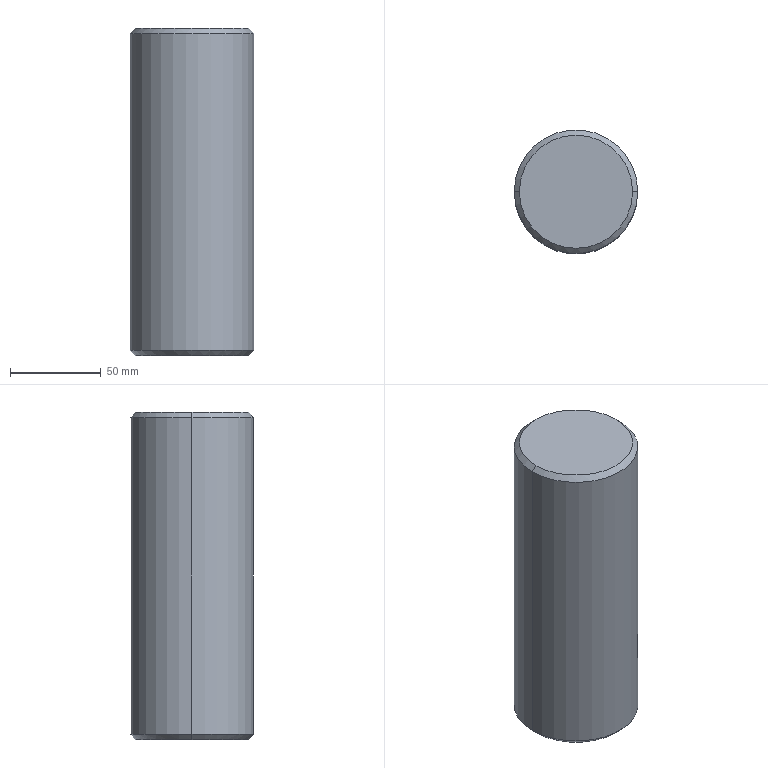Part | SolidWorks | features BaseBody 1 | 1 solid | 12 faces | box 68 x 68 x 180 mm | volume 648919 mm3 | cone 6 | cylinder 4 | plane 2 | commonest cylinder face diameters 10.5 x2 68 x2
STEP:
#1=CARTESIAN_POINT('',(214.75,-51.999,-390.5));
#2=VERTEX_POINT('',#1);
#3=CARTESIAN_POINT('',(225.25,-51.999,-390.5));
#4=VERTEX_POINT('',#3);
#5=CARTESIAN_POINT('',(220.,-51.999,-390.5));
#6=DIRECTION('',(0.,0.,1.));
#7=DIRECTION('',(1.,0.,0.));
#8=AXIS2_PLACEMENT_3D('',#5,#6,#7);
#9=CIRCLE('',#8,5.25);
#10=EDGE_CURVE('',#2,#4,#9,.T.);
#11=ORIENTED_EDGE('',*,*,#10,.F.);
#12=CARTESIAN_POINT('',(214.75,-51.999,-355.5));
#13=VERTEX_POINT('',#12);
#14=CARTESIAN_POINT('',(214.75,-51.999,-390.5));
#15=DIRECTION('',(0.,0.,1.));
#16=VECTOR('',#15,1000.);
#17=LINE('',#14,#16);
#18=EDGE_CURVE('',#2,#13,#17,.T.);
#19=ORIENTED_EDGE('',*,*,#18,.T.);
#20=CARTESIAN_POINT('',(225.25,-51.999,-355.5));
#21=VERTEX_POINT('',#20);
#22=CARTESIAN_POINT('',(220.,-51.999,-355.5));
#23=DIRECTION('',(0.,0.,1.));
#24=DIRECTION('',(1.,0.,0.));
#25=AXIS2_PLACEMENT_3D('',#22,#23,#24);
#26=CIRCLE('',#25,5.25);
#27=EDGE_CURVE('',#13,#21,#26,.T.);
#28=ORIENTED_EDGE('',*,*,#27,.T.);
#29=CARTESIAN_POINT('',(225.25,-51.999,-390.5));
#30=DIRECTION('',(0.,0.,1.));
#31=VECTOR('',#30,1000.);
#32=LINE('',#29,#31);
#33=EDGE_CURVE('',#4,#21,#32,.T.);
#34=ORIENTED_EDGE('',*,*,#33,.F.);
#35=EDGE_LOOP('',(#11,#19,#28,#34));
#36=FACE_OUTER_BOUND('',#35,.T.);
#37=CARTESIAN_POINT('',(220.,-51.999,-390.5));
#38=DIRECTION('',(0.,0.,1.));
#39=DIRECTION('',(1.,0.,0.));
#40=AXIS2_PLACEMENT_3D('',#37,#38,#39);
#41=CYLINDRICAL_SURFACE('',#40,5.25);
#42=ADVANCED_FACE('',(#36),#41,.F.);
#43=CARTESIAN_POINT('',(220.,-51.999,-352.345));
#44=VERTEX_POINT('',#43);
#45=CARTESIAN_POINT('',(214.75,-51.999,-355.5));
#46=DIRECTION('',(-0.8572,0.,-0.515));
#47=VECTOR('',#46,1000.);
#48=LINE('',#45,#47);
#49=EDGE_CURVE('',#44,#13,#48,.T.);
#50=ORIENTED_EDGE('',*,*,#49,.F.);
#51=CARTESIAN_POINT('',(225.25,-51.999,-355.5));
#52=DIRECTION('',(0.8572,0.,-0.515));
#53=VECTOR('',#52,1000.);
#54=LINE('',#51,#53);
#55=EDGE_CURVE('',#44,#21,#54,.T.);
#56=ORIENTED_EDGE('',*,*,#55,.T.);
#57=ORIENTED_EDGE('',*,*,#27,.F.);
#58=EDGE_LOOP('',(#50,#56,#57));
#59=FACE_OUTER_BOUND('',#58,.T.);
#60=CARTESIAN_POINT('',(220.,-51.999,-355.5));
#61=DIRECTION('',(0.,0.,-1.));
#62=DIRECTION('',(-1.,0.,0.));
#63=AXIS2_PLACEMENT_3D('',#60,#61,#62);
#64=CONICAL_SURFACE('',#63,5.25,1.03);
#65=ADVANCED_FACE('',(#59),#64,.F.);
#66=CARTESIAN_POINT('',(251.172,-51.999,-210.5));
#67=VERTEX_POINT('',#66);
#68=CARTESIAN_POINT('',(188.828,-51.999,-210.5));
#69=VERTEX_POINT('',#68);
#70=CARTESIAN_POINT('',(220.,-51.999,-210.5));
#71=DIRECTION('',(0.,0.,1.));
#72=DIRECTION('',(1.,0.,0.));
#73=AXIS2_PLACEMENT_3D('',#70,#71,#72);
#74=CIRCLE('',#73,31.172);
#75=EDGE_CURVE('',#67,#69,#74,.T.);
#76=ORIENTED_EDGE('',*,*,#75,.F.);
#77=CARTESIAN_POINT('',(254.,-51.999,-213.328));
#78=VERTEX_POINT('',#77);
#79=CARTESIAN_POINT('',(252.586,-51.999,-211.914));
#80=DIRECTION('',(0.7071,0.,-0.7071));
#81=VECTOR('',#80,1000.);
#82=LINE('',#79,#81);
#83=EDGE_CURVE('',#67,#78,#82,.T.);
#84=ORIENTED_EDGE('',*,*,#83,.T.);
#85=CARTESIAN_POINT('',(186.,-51.999,-213.328));
#86=VERTEX_POINT('',#85);
#87=CARTESIAN_POINT('',(220.,-51.999,-213.328));
#88=DIRECTION('',(0.,0.,-1.));
#89=DIRECTION('',(-1.,0.,0.));
#90=AXIS2_PLACEMENT_3D('',#87,#88,#89);
#91=CIRCLE('',#90,34.);
#92=EDGE_CURVE('',#86,#78,#91,.T.);
#93=ORIENTED_EDGE('',*,*,#92,.F.);
#94=CARTESIAN_POINT('',(187.414,-51.999,-211.914));
#95=DIRECTION('',(-0.7071,0.,-0.7071));
#96=VECTOR('',#95,1000.);
#97=LINE('',#94,#96);
#98=EDGE_CURVE('',#69,#86,#97,.T.);
#99=ORIENTED_EDGE('',*,*,#98,.F.);
#100=EDGE_LOOP('',(#76,#84,#93,#99));
#101=FACE_OUTER_BOUND('',#100,.T.);
#102=CARTESIAN_POINT('',(220.,-51.999,-211.914));
#103=DIRECTION('',(0.,0.,-1.));
#104=DIRECTION('',(-1.,0.,0.));
#105=AXIS2_PLACEMENT_3D('',#102,#103,#104);
#106=CONICAL_SURFACE('',#105,32.586,0.7854);
#107=ADVANCED_FACE('',(#101),#106,.T.);
#108=CARTESIAN_POINT('',(188.828,-51.999,-390.5));
#109=VERTEX_POINT('',#108);
#110=CARTESIAN_POINT('',(251.172,-51.999,-390.5));
#111=VERTEX_POINT('',#110);
#112=CARTESIAN_POINT('',(220.,-51.999,-390.5));
#113=DIRECTION('',(0.,0.,-1.));
#114=DIRECTION('',(1.,0.,0.));
#115=AXIS2_PLACEMENT_3D('',#112,#113,#114);
#116=CIRCLE('',#115,31.172);
#117=EDGE_CURVE('',#109,#111,#116,.T.);
#118=ORIENTED_EDGE('',*,*,#117,.F.);
#119=CARTESIAN_POINT('',(186.,-51.999,-387.672));
#120=VERTEX_POINT('',#119);
#121=CARTESIAN_POINT('',(185.414,-51.999,-387.086));
#122=DIRECTION('',(-0.7071,0.,0.7071));
#123=VECTOR('',#122,1000.);
#124=LINE('',#121,#123);
#125=EDGE_CURVE('',#109,#120,#124,.T.);
#126=ORIENTED_EDGE('',*,*,#125,.T.);
#127=CARTESIAN_POINT('',(254.,-51.999,-387.672));
#128=VERTEX_POINT('',#127);
#129=CARTESIAN_POINT('',(220.,-51.999,-387.672));
#130=DIRECTION('',(0.,0.,1.));
#131=DIRECTION('',(1.,0.,0.));
#132=AXIS2_PLACEMENT_3D('',#129,#130,#131);
#133=CIRCLE('',#132,34.);
#134=EDGE_CURVE('',#128,#120,#133,.T.);
#135=ORIENTED_EDGE('',*,*,#134,.F.);
#136=CARTESIAN_POINT('',(254.586,-51.999,-387.086));
#137=DIRECTION('',(0.7071,0.,0.7071));
#138=VECTOR('',#137,1000.);
#139=LINE('',#136,#138);
#140=EDGE_CURVE('',#111,#128,#139,.T.);
#141=ORIENTED_EDGE('',*,*,#140,.F.);
#142=EDGE_LOOP('',(#118,#126,#135,#141));
#143=FACE_OUTER_BOUND('',#142,.T.);
#144=CARTESIAN_POINT('',(220.,-51.999,-387.086));
#145=DIRECTION('',(0.,0.,1.));
#146=DIRECTION('',(1.,0.,0.));
#147=AXIS2_PLACEMENT_3D('',#144,#145,#146);
#148=CONICAL_SURFACE('',#147,34.586,0.7854);
#149=ADVANCED_FACE('',(#143),#148,.T.);
#150=ORIENTED_EDGE('',*,*,#92,.T.);
#151=CARTESIAN_POINT('',(254.,-51.999,-210.5));
#152=DIRECTION('',(0.,0.,-1.));
#153=VECTOR('',#152,1000.);
#154=LINE('',#151,#153);
#155=EDGE_CURVE('',#78,#128,#154,.T.);
#156=ORIENTED_EDGE('',*,*,#155,.T.);
#157=ORIENTED_EDGE('',*,*,#134,.T.);
#158=CARTESIAN_POINT('',(186.,-51.999,-210.5));
#159=DIRECTION('',(0.,0.,-1.));
#160=VECTOR('',#159,1000.);
#161=LINE('',#158,#160);
#162=EDGE_CURVE('',#86,#120,#161,.T.);
#163=ORIENTED_EDGE('',*,*,#162,.F.);
#164=EDGE_LOOP('',(#150,#156,#157,#163));
#165=FACE_OUTER_BOUND('',#164,.T.);
#166=CARTESIAN_POINT('',(220.,-51.999,-210.5));
#167=DIRECTION('',(0.,0.,-1.));
#168=DIRECTION('',(-1.,0.,0.));
#169=AXIS2_PLACEMENT_3D('',#166,#167,#168);
#170=CYLINDRICAL_SURFACE('',#169,34.);
#171=ADVANCED_FACE('',(#165),#170,.T.);
#172=ORIENTED_EDGE('',*,*,#155,.F.);
#173=CARTESIAN_POINT('',(220.,-51.999,-213.328));
#174=DIRECTION('',(0.,0.,-1.));
#175=DIRECTION('',(-1.,0.,0.));
#176=AXIS2_PLACEMENT_3D('',#173,#174,#175);
#177=CIRCLE('',#176,34.);
#178=EDGE_CURVE('',#78,#86,#177,.T.);
#179=ORIENTED_EDGE('',*,*,#178,.T.);
#180=ORIENTED_EDGE('',*,*,#162,.T.);
#181=CARTESIAN_POINT('',(220.,-51.999,-387.672));
#182=DIRECTION('',(0.,0.,1.));
#183=DIRECTION('',(1.,0.,0.));
#184=AXIS2_PLACEMENT_3D('',#181,#182,#183);
#185=CIRCLE('',#184,34.);
#186=EDGE_CURVE('',#120,#128,#185,.T.);
#187=ORIENTED_EDGE('',*,*,#186,.T.);
#188=EDGE_LOOP('',(#172,#179,#180,#187));
#189=FACE_OUTER_BOUND('',#188,.T.);
#190=CARTESIAN_POINT('',(220.,-51.999,-210.5));
#191=DIRECTION('',(0.,0.,-1.));
#192=DIRECTION('',(-1.,0.,0.));
#193=AXIS2_PLACEMENT_3D('',#190,#191,#192);
#194=CYLINDRICAL_SURFACE('',#193,34.);
#195=ADVANCED_FACE('',(#189),#194,.T.);
#196=CARTESIAN_POINT('',(220.,-51.999,-210.5));
#197=DIRECTION('',(0.,0.,1.));
#198=DIRECTION('',(1.,0.,0.));
#199=AXIS2_PLACEMENT_3D('',#196,#197,#198);
#200=CIRCLE('',#199,31.172);
#201=EDGE_CURVE('',#69,#67,#200,.T.);
#202=ORIENTED_EDGE('',*,*,#201,.T.);
#203=ORIENTED_EDGE('',*,*,#75,.T.);
#204=EDGE_LOOP('',(#202,#203));
#205=FACE_OUTER_BOUND('',#204,.T.);
#206=CARTESIAN_POINT('',(220.,-51.999,-210.5));
#207=DIRECTION('',(0.,0.,1.));
#208=DIRECTION('',(1.,0.,0.));
#209=AXIS2_PLACEMENT_3D('',#206,#207,#208);
#210=PLANE('',#209);
#211=ADVANCED_FACE('',(#205),#210,.T.);
#212=CARTESIAN_POINT('',(220.,-51.999,-390.5));
#213=DIRECTION('',(0.,0.,1.));
#214=DIRECTION('',(1.,0.,0.));
#215=AXIS2_PLACEMENT_3D('',#212,#213,#214);
#216=CIRCLE('',#215,5.25);
#217=EDGE_CURVE('',#4,#2,#216,.T.);
#218=ORIENTED_EDGE('',*,*,#217,.T.);
#219=ORIENTED_EDGE('',*,*,#10,.T.);
#220=EDGE_LOOP('',(#218,#219));
#221=FACE_BOUND('',#220,.T.);
#222=CARTESIAN_POINT('',(220.,-51.999,-390.5));
#223=DIRECTION('',(0.,0.,-1.));
#224=DIRECTION('',(1.,0.,0.));
#225=AXIS2_PLACEMENT_3D('',#222,#223,#224);
#226=CIRCLE('',#225,31.172);
#227=EDGE_CURVE('',#111,#109,#226,.T.);
#228=ORIENTED_EDGE('',*,*,#227,.T.);
#229=ORIENTED_EDGE('',*,*,#117,.T.);
#230=EDGE_LOOP('',(#228,#229));
#231=FACE_OUTER_BOUND('',#230,.T.);
#232=CARTESIAN_POINT('',(220.,-51.999,-390.5));
#233=DIRECTION('',(0.,0.,1.));
#234=DIRECTION('',(1.,0.,0.));
#235=AXIS2_PLACEMENT_3D('',#232,#233,#234);
#236=PLANE('',#235);
#237=ADVANCED_FACE('',(#221,#231),#236,.F.);
#238=ORIENTED_EDGE('',*,*,#125,.F.);
#239=ORIENTED_EDGE('',*,*,#227,.F.);
#240=ORIENTED_EDGE('',*,*,#140,.T.);
#241=ORIENTED_EDGE('',*,*,#186,.F.);
#242=EDGE_LOOP('',(#238,#239,#240,#241));
#243=FACE_OUTER_BOUND('',#242,.T.);
#244=CARTESIAN_POINT('',(220.,-51.999,-387.086));
#245=DIRECTION('',(0.,0.,1.));
#246=DIRECTION('',(1.,0.,0.));
#247=AXIS2_PLACEMENT_3D('',#244,#245,#246);
#248=CONICAL_SURFACE('',#247,34.586,0.7854);
#249=ADVANCED_FACE('',(#243),#248,.T.);
#250=ORIENTED_EDGE('',*,*,#83,.F.);
#251=ORIENTED_EDGE('',*,*,#201,.F.);
#252=ORIENTED_EDGE('',*,*,#98,.T.);
#253=ORIENTED_EDGE('',*,*,#178,.F.);
#254=EDGE_LOOP('',(#250,#251,#252,#253));
#255=FACE_OUTER_BOUND('',#254,.T.);
#256=CARTESIAN_POINT('',(220.,-51.999,-211.914));
#257=DIRECTION('',(0.,0.,-1.));
#258=DIRECTION('',(-1.,0.,0.));
#259=AXIS2_PLACEMENT_3D('',#256,#257,#258);
#260=CONICAL_SURFACE('',#259,32.586,0.7854);
#261=ADVANCED_FACE('',(#255),#260,.T.);
#262=ORIENTED_EDGE('',*,*,#55,.F.);
#263=ORIENTED_EDGE('',*,*,#49,.T.);
#264=CARTESIAN_POINT('',(220.,-51.999,-355.5));
#265=DIRECTION('',(0.,0.,1.));
#266=DIRECTION('',(1.,0.,0.));
#267=AXIS2_PLACEMENT_3D('',#264,#265,#266);
#268=CIRCLE('',#267,5.25);
#269=EDGE_CURVE('',#21,#13,#268,.T.);
#270=ORIENTED_EDGE('',*,*,#269,.F.);
#271=EDGE_LOOP('',(#262,#263,#270));
#272=FACE_OUTER_BOUND('',#271,.T.);
#273=CARTESIAN_POINT('',(220.,-51.999,-355.5));
#274=DIRECTION('',(0.,0.,-1.));
#275=DIRECTION('',(-1.,0.,0.));
#276=AXIS2_PLACEMENT_3D('',#273,#274,#275);
#277=CONICAL_SURFACE('',#276,5.25,1.03);
#278=ADVANCED_FACE('',(#272),#277,.F.);
#279=ORIENTED_EDGE('',*,*,#18,.F.);
#280=ORIENTED_EDGE('',*,*,#217,.F.);
#281=ORIENTED_EDGE('',*,*,#33,.T.);
#282=ORIENTED_EDGE('',*,*,#269,.T.);
#283=EDGE_LOOP('',(#279,#280,#281,#282));
#284=FACE_OUTER_BOUND('',#283,.T.);
#285=CARTESIAN_POINT('',(220.,-51.999,-390.5));
#286=DIRECTION('',(0.,0.,1.));
#287=DIRECTION('',(1.,0.,0.));
#288=AXIS2_PLACEMENT_3D('',#285,#286,#287);
#289=CYLINDRICAL_SURFACE('',#288,5.25);
#290=ADVANCED_FACE('',(#284),#289,.F.);
#291=CLOSED_SHELL('',(#42,#65,#107,#149,#171,#195,#211,#237,#249,#261,#278,#290));
#292=MANIFOLD_SOLID_BREP('',#291);
#293=CARTESIAN_POINT('',(0.,0.,0.));
#294=DIRECTION('',(0.,0.,1.));
#295=DIRECTION('',(1.,0.,0.));
#296=AXIS2_PLACEMENT_3D('',#293,#294,#295);
#297=(LENGTH_UNIT()NAMED_UNIT(*)SI_UNIT(.MILLI.,.METRE.));
#298=UNCERTAINTY_MEASURE_WITH_UNIT(LENGTH_MEASURE(0.00001),#297,'','');
#299=(NAMED_UNIT(*)PLANE_ANGLE_UNIT()SI_UNIT($,.RADIAN.));
#300=(NAMED_UNIT(*)SI_UNIT($,.STERADIAN.)SOLID_ANGLE_UNIT());
#301=(GEOMETRIC_REPRESENTATION_CONTEXT(3)GLOBAL_UNCERTAINTY_ASSIGNED_CONTEXT((#298))GLOBAL_UNIT_ASSIGNED_CONTEXT((#297,#299,#300))REPRESENTATION_CONTEXT('',''));
#302=ADVANCED_BREP_SHAPE_REPRESENTATION('',(#292,#296),#301);